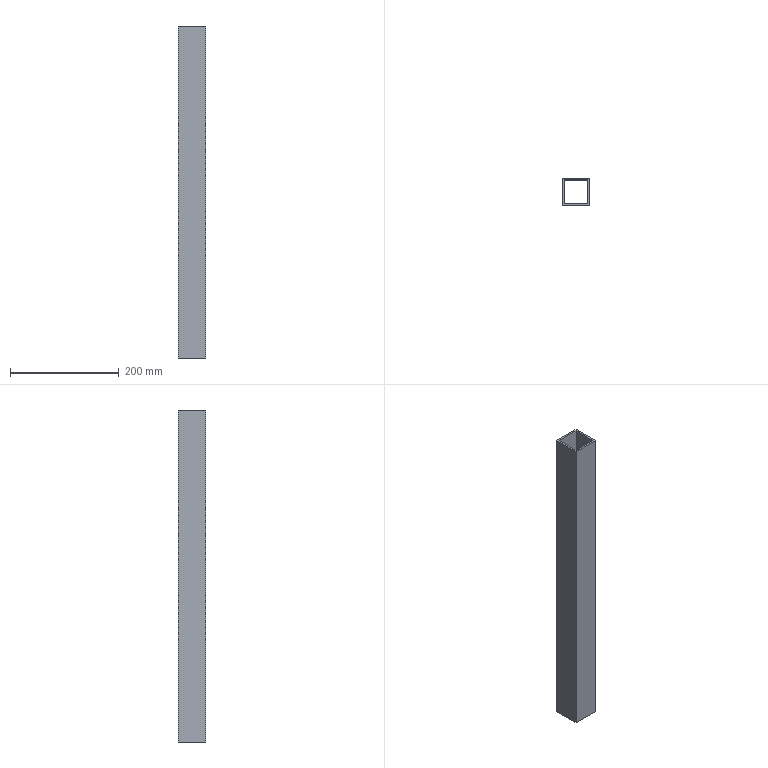Part | STEP file | BCC3 H19_2 | 1 solid | 10 faces | box 50 x 50 x 610 mm | volume 344040 mm3 | plane 10
STEP:
#1=CARTESIAN_POINT('',(0.,0.,0.));
#2=DIRECTION('',(0.,0.,1.));
#3=DIRECTION('',(1.,0.,0.));
#4=AXIS2_PLACEMENT_3D('',#1,#2,#3);
#5=CARTESIAN_POINT('',(-25.,25.,305.));
#6=VERTEX_POINT('',#5);
#7=CARTESIAN_POINT('',(-25.,-25.,305.));
#8=VERTEX_POINT('',#7);
#9=CARTESIAN_POINT('',(-25.,25.,305.));
#10=DIRECTION('',(0.,-1.,0.));
#11=VECTOR('',#10,1.);
#12=LINE('',#9,#11);
#13=CARTESIAN_POINT('',(0.,0.,305.));
#14=DIRECTION('',(0.,0.,1.));
#15=DIRECTION('',(1.,0.,0.));
#16=AXIS2_PLACEMENT_3D('',#13,#14,#15);
#17=PLANE('',#16);
#18=CARTESIAN_POINT('',(-25.,25.));
#19=DIRECTION('',(0.,-1.));
#20=VECTOR('',#19,1.);
#21=LINE('',#18,#20);
#22=(GEOMETRIC_REPRESENTATION_CONTEXT(2)PARAMETRIC_REPRESENTATION_CONTEXT()REPRESENTATION_CONTEXT('',''));
#23=DEFINITIONAL_REPRESENTATION('',(#21),#22);
#24=PCURVE('',#17,#23);
#25=CARTESIAN_POINT('',(-25.,25.,305.));
#26=DIRECTION('',(1.,0.,0.));
#27=DIRECTION('',(0.,1.,0.));
#28=AXIS2_PLACEMENT_3D('',#25,#26,#27);
#29=PLANE('',#28);
#30=CARTESIAN_POINT('',(0.,0.));
#31=DIRECTION('',(-1.,0.));
#32=VECTOR('',#31,1.);
#33=LINE('',#30,#32);
#34=(GEOMETRIC_REPRESENTATION_CONTEXT(2)PARAMETRIC_REPRESENTATION_CONTEXT()REPRESENTATION_CONTEXT('',''));
#35=DEFINITIONAL_REPRESENTATION('',(#33),#34);
#36=PCURVE('',#29,#35);
#37=SURFACE_CURVE('',#12,(#24,#36),.PCURVE_S1.);
#38=EDGE_CURVE('',#6,#8,#37,.T.);
#39=ORIENTED_EDGE('',*,*,#38,.T.);
#40=CARTESIAN_POINT('',(25.,-25.,305.));
#41=VERTEX_POINT('',#40);
#42=CARTESIAN_POINT('',(-25.,-25.,305.));
#43=DIRECTION('',(1.,0.,0.));
#44=VECTOR('',#43,1.);
#45=LINE('',#42,#44);
#46=CARTESIAN_POINT('',(-25.,-25.));
#47=DIRECTION('',(1.,0.));
#48=VECTOR('',#47,1.);
#49=LINE('',#46,#48);
#50=(GEOMETRIC_REPRESENTATION_CONTEXT(2)PARAMETRIC_REPRESENTATION_CONTEXT()REPRESENTATION_CONTEXT('',''));
#51=DEFINITIONAL_REPRESENTATION('',(#49),#50);
#52=PCURVE('',#17,#51);
#53=CARTESIAN_POINT('',(-25.,-25.,305.));
#54=DIRECTION('',(0.,1.,0.));
#55=DIRECTION('',(0.,0.,1.));
#56=AXIS2_PLACEMENT_3D('',#53,#54,#55);
#57=PLANE('',#56);
#58=CARTESIAN_POINT('',(0.,0.));
#59=DIRECTION('',(0.,1.));
#60=VECTOR('',#59,1.);
#61=LINE('',#58,#60);
#62=(GEOMETRIC_REPRESENTATION_CONTEXT(2)PARAMETRIC_REPRESENTATION_CONTEXT()REPRESENTATION_CONTEXT('',''));
#63=DEFINITIONAL_REPRESENTATION('',(#61),#62);
#64=PCURVE('',#57,#63);
#65=SURFACE_CURVE('',#45,(#52,#64),.PCURVE_S1.);
#66=EDGE_CURVE('',#8,#41,#65,.T.);
#67=ORIENTED_EDGE('',*,*,#66,.T.);
#68=CARTESIAN_POINT('',(25.,25.,305.));
#69=VERTEX_POINT('',#68);
#70=CARTESIAN_POINT('',(25.,25.,305.));
#71=DIRECTION('',(0.,1.,0.));
#72=VECTOR('',#71,1.);
#73=LINE('',#70,#72);
#74=CARTESIAN_POINT('',(25.,25.));
#75=DIRECTION('',(0.,1.));
#76=VECTOR('',#75,1.);
#77=LINE('',#74,#76);
#78=(GEOMETRIC_REPRESENTATION_CONTEXT(2)PARAMETRIC_REPRESENTATION_CONTEXT()REPRESENTATION_CONTEXT('',''));
#79=DEFINITIONAL_REPRESENTATION('',(#77),#78);
#80=PCURVE('',#17,#79);
#81=CARTESIAN_POINT('',(25.,25.,305.));
#82=DIRECTION('',(-1.,0.,0.));
#83=DIRECTION('',(0.,-1.,0.));
#84=AXIS2_PLACEMENT_3D('',#81,#82,#83);
#85=PLANE('',#84);
#86=CARTESIAN_POINT('',(0.,0.));
#87=DIRECTION('',(-1.,0.));
#88=VECTOR('',#87,1.);
#89=LINE('',#86,#88);
#90=(GEOMETRIC_REPRESENTATION_CONTEXT(2)PARAMETRIC_REPRESENTATION_CONTEXT()REPRESENTATION_CONTEXT('',''));
#91=DEFINITIONAL_REPRESENTATION('',(#89),#90);
#92=PCURVE('',#85,#91);
#93=SURFACE_CURVE('',#73,(#80,#92),.PCURVE_S1.);
#94=EDGE_CURVE('',#41,#69,#93,.T.);
#95=ORIENTED_EDGE('',*,*,#94,.T.);
#96=CARTESIAN_POINT('',(-25.,25.,305.));
#97=DIRECTION('',(-1.,0.,0.));
#98=VECTOR('',#97,1.);
#99=LINE('',#96,#98);
#100=CARTESIAN_POINT('',(-25.,25.));
#101=DIRECTION('',(-1.,0.));
#102=VECTOR('',#101,1.);
#103=LINE('',#100,#102);
#104=(GEOMETRIC_REPRESENTATION_CONTEXT(2)PARAMETRIC_REPRESENTATION_CONTEXT()REPRESENTATION_CONTEXT('',''));
#105=DEFINITIONAL_REPRESENTATION('',(#103),#104);
#106=PCURVE('',#17,#105);
#107=CARTESIAN_POINT('',(-25.,25.,305.));
#108=DIRECTION('',(0.,-1.,0.));
#109=DIRECTION('',(0.,0.,-1.));
#110=AXIS2_PLACEMENT_3D('',#107,#108,#109);
#111=PLANE('',#110);
#112=CARTESIAN_POINT('',(0.,0.));
#113=DIRECTION('',(0.,-1.));
#114=VECTOR('',#113,1.);
#115=LINE('',#112,#114);
#116=(GEOMETRIC_REPRESENTATION_CONTEXT(2)PARAMETRIC_REPRESENTATION_CONTEXT()REPRESENTATION_CONTEXT('',''));
#117=DEFINITIONAL_REPRESENTATION('',(#115),#116);
#118=PCURVE('',#111,#117);
#119=SURFACE_CURVE('',#99,(#106,#118),.PCURVE_S1.);
#120=EDGE_CURVE('',#69,#6,#119,.T.);
#121=ORIENTED_EDGE('',*,*,#120,.T.);
#122=EDGE_LOOP('',(#39,#67,#95,#121));
#123=FACE_BOUND('',#122,.T.);
#124=CARTESIAN_POINT('',(-22.,-22.,305.));
#125=VERTEX_POINT('',#124);
#126=CARTESIAN_POINT('',(22.,-22.,305.));
#127=VERTEX_POINT('',#126);
#128=CARTESIAN_POINT('',(-22.,-22.,305.));
#129=DIRECTION('',(1.,0.,0.));
#130=VECTOR('',#129,1.);
#131=LINE('',#128,#130);
#132=CARTESIAN_POINT('',(-22.,-22.));
#133=DIRECTION('',(1.,0.));
#134=VECTOR('',#133,1.);
#135=LINE('',#132,#134);
#136=(GEOMETRIC_REPRESENTATION_CONTEXT(2)PARAMETRIC_REPRESENTATION_CONTEXT()REPRESENTATION_CONTEXT('',''));
#137=DEFINITIONAL_REPRESENTATION('',(#135),#136);
#138=PCURVE('',#17,#137);
#139=CARTESIAN_POINT('',(-22.,-22.,305.));
#140=DIRECTION('',(0.,1.,0.));
#141=DIRECTION('',(-1.,0.,0.));
#142=AXIS2_PLACEMENT_3D('',#139,#140,#141);
#143=PLANE('',#142);
#144=CARTESIAN_POINT('',(0.,0.));
#145=DIRECTION('',(-1.,0.));
#146=VECTOR('',#145,1.);
#147=LINE('',#144,#146);
#148=(GEOMETRIC_REPRESENTATION_CONTEXT(2)PARAMETRIC_REPRESENTATION_CONTEXT()REPRESENTATION_CONTEXT('',''));
#149=DEFINITIONAL_REPRESENTATION('',(#147),#148);
#150=PCURVE('',#143,#149);
#151=SURFACE_CURVE('',#131,(#138,#150),.PCURVE_S1.);
#152=EDGE_CURVE('',#125,#127,#151,.T.);
#153=ORIENTED_EDGE('',*,*,#152,.F.);
#154=CARTESIAN_POINT('',(-22.,22.,305.));
#155=VERTEX_POINT('',#154);
#156=CARTESIAN_POINT('',(-22.,22.,305.));
#157=DIRECTION('',(0.,-1.,0.));
#158=VECTOR('',#157,1.);
#159=LINE('',#156,#158);
#160=CARTESIAN_POINT('',(-22.,22.));
#161=DIRECTION('',(0.,-1.));
#162=VECTOR('',#161,1.);
#163=LINE('',#160,#162);
#164=(GEOMETRIC_REPRESENTATION_CONTEXT(2)PARAMETRIC_REPRESENTATION_CONTEXT()REPRESENTATION_CONTEXT('',''));
#165=DEFINITIONAL_REPRESENTATION('',(#163),#164);
#166=PCURVE('',#17,#165);
#167=CARTESIAN_POINT('',(-22.,22.,305.));
#168=DIRECTION('',(1.,0.,0.));
#169=DIRECTION('',(0.,1.,0.));
#170=AXIS2_PLACEMENT_3D('',#167,#168,#169);
#171=PLANE('',#170);
#172=CARTESIAN_POINT('',(0.,0.));
#173=DIRECTION('',(-1.,0.));
#174=VECTOR('',#173,1.);
#175=LINE('',#172,#174);
#176=(GEOMETRIC_REPRESENTATION_CONTEXT(2)PARAMETRIC_REPRESENTATION_CONTEXT()REPRESENTATION_CONTEXT('',''));
#177=DEFINITIONAL_REPRESENTATION('',(#175),#176);
#178=PCURVE('',#171,#177);
#179=SURFACE_CURVE('',#159,(#166,#178),.PCURVE_S1.);
#180=EDGE_CURVE('',#155,#125,#179,.T.);
#181=ORIENTED_EDGE('',*,*,#180,.F.);
#182=CARTESIAN_POINT('',(22.,22.,305.));
#183=VERTEX_POINT('',#182);
#184=CARTESIAN_POINT('',(-22.,22.,305.));
#185=DIRECTION('',(-1.,0.,0.));
#186=VECTOR('',#185,1.);
#187=LINE('',#184,#186);
#188=CARTESIAN_POINT('',(-22.,22.));
#189=DIRECTION('',(-1.,0.));
#190=VECTOR('',#189,1.);
#191=LINE('',#188,#190);
#192=(GEOMETRIC_REPRESENTATION_CONTEXT(2)PARAMETRIC_REPRESENTATION_CONTEXT()REPRESENTATION_CONTEXT('',''));
#193=DEFINITIONAL_REPRESENTATION('',(#191),#192);
#194=PCURVE('',#17,#193);
#195=CARTESIAN_POINT('',(-22.,22.,305.));
#196=DIRECTION('',(0.,-1.,0.));
#197=DIRECTION('',(0.,0.,-1.));
#198=AXIS2_PLACEMENT_3D('',#195,#196,#197);
#199=PLANE('',#198);
#200=CARTESIAN_POINT('',(0.,0.));
#201=DIRECTION('',(0.,-1.));
#202=VECTOR('',#201,1.);
#203=LINE('',#200,#202);
#204=(GEOMETRIC_REPRESENTATION_CONTEXT(2)PARAMETRIC_REPRESENTATION_CONTEXT()REPRESENTATION_CONTEXT('',''));
#205=DEFINITIONAL_REPRESENTATION('',(#203),#204);
#206=PCURVE('',#199,#205);
#207=SURFACE_CURVE('',#187,(#194,#206),.PCURVE_S1.);
#208=EDGE_CURVE('',#183,#155,#207,.T.);
#209=ORIENTED_EDGE('',*,*,#208,.F.);
#210=CARTESIAN_POINT('',(22.,22.,305.));
#211=DIRECTION('',(0.,1.,0.));
#212=VECTOR('',#211,1.);
#213=LINE('',#210,#212);
#214=CARTESIAN_POINT('',(22.,22.));
#215=DIRECTION('',(0.,1.));
#216=VECTOR('',#215,1.);
#217=LINE('',#214,#216);
#218=(GEOMETRIC_REPRESENTATION_CONTEXT(2)PARAMETRIC_REPRESENTATION_CONTEXT()REPRESENTATION_CONTEXT('',''));
#219=DEFINITIONAL_REPRESENTATION('',(#217),#218);
#220=PCURVE('',#17,#219);
#221=CARTESIAN_POINT('',(22.,22.,305.));
#222=DIRECTION('',(-1.,0.,0.));
#223=DIRECTION('',(0.,-1.,0.));
#224=AXIS2_PLACEMENT_3D('',#221,#222,#223);
#225=PLANE('',#224);
#226=CARTESIAN_POINT('',(0.,0.));
#227=DIRECTION('',(-1.,0.));
#228=VECTOR('',#227,1.);
#229=LINE('',#226,#228);
#230=(GEOMETRIC_REPRESENTATION_CONTEXT(2)PARAMETRIC_REPRESENTATION_CONTEXT()REPRESENTATION_CONTEXT('',''));
#231=DEFINITIONAL_REPRESENTATION('',(#229),#230);
#232=PCURVE('',#225,#231);
#233=SURFACE_CURVE('',#213,(#220,#232),.PCURVE_S1.);
#234=EDGE_CURVE('',#127,#183,#233,.T.);
#235=ORIENTED_EDGE('',*,*,#234,.F.);
#236=EDGE_LOOP('',(#153,#181,#209,#235));
#237=FACE_BOUND('',#236,.T.);
#238=ADVANCED_FACE('',(#123,#237),#17,.T.);
#239=CARTESIAN_POINT('',(-25.,25.,-305.));
#240=VERTEX_POINT('',#239);
#241=CARTESIAN_POINT('',(-25.,-25.,-305.));
#242=VERTEX_POINT('',#241);
#243=CARTESIAN_POINT('',(-25.,25.,-305.));
#244=DIRECTION('',(0.,-1.,0.));
#245=VECTOR('',#244,1.);
#246=LINE('',#243,#245);
#247=CARTESIAN_POINT('',(0.,0.,-305.));
#248=DIRECTION('',(0.,0.,1.));
#249=DIRECTION('',(1.,0.,0.));
#250=AXIS2_PLACEMENT_3D('',#247,#248,#249);
#251=PLANE('',#250);
#252=CARTESIAN_POINT('',(-25.,25.));
#253=DIRECTION('',(0.,-1.));
#254=VECTOR('',#253,1.);
#255=LINE('',#252,#254);
#256=(GEOMETRIC_REPRESENTATION_CONTEXT(2)PARAMETRIC_REPRESENTATION_CONTEXT()REPRESENTATION_CONTEXT('',''));
#257=DEFINITIONAL_REPRESENTATION('',(#255),#256);
#258=PCURVE('',#251,#257);
#259=CARTESIAN_POINT('',(0.,-610.));
#260=DIRECTION('',(-1.,0.));
#261=VECTOR('',#260,1.);
#262=LINE('',#259,#261);
#263=(GEOMETRIC_REPRESENTATION_CONTEXT(2)PARAMETRIC_REPRESENTATION_CONTEXT()REPRESENTATION_CONTEXT('',''));
#264=DEFINITIONAL_REPRESENTATION('',(#262),#263);
#265=PCURVE('',#29,#264);
#266=SURFACE_CURVE('',#246,(#258,#265),.PCURVE_S1.);
#267=EDGE_CURVE('',#240,#242,#266,.T.);
#268=ORIENTED_EDGE('',*,*,#267,.F.);
#269=CARTESIAN_POINT('',(25.,25.,-305.));
#270=VERTEX_POINT('',#269);
#271=CARTESIAN_POINT('',(-25.,25.,-305.));
#272=DIRECTION('',(-1.,0.,0.));
#273=VECTOR('',#272,1.);
#274=LINE('',#271,#273);
#275=CARTESIAN_POINT('',(-25.,25.));
#276=DIRECTION('',(-1.,0.));
#277=VECTOR('',#276,1.);
#278=LINE('',#275,#277);
#279=(GEOMETRIC_REPRESENTATION_CONTEXT(2)PARAMETRIC_REPRESENTATION_CONTEXT()REPRESENTATION_CONTEXT('',''));
#280=DEFINITIONAL_REPRESENTATION('',(#278),#279);
#281=PCURVE('',#251,#280);
#282=CARTESIAN_POINT('',(610.,0.));
#283=DIRECTION('',(0.,-1.));
#284=VECTOR('',#283,1.);
#285=LINE('',#282,#284);
#286=(GEOMETRIC_REPRESENTATION_CONTEXT(2)PARAMETRIC_REPRESENTATION_CONTEXT()REPRESENTATION_CONTEXT('',''));
#287=DEFINITIONAL_REPRESENTATION('',(#285),#286);
#288=PCURVE('',#111,#287);
#289=SURFACE_CURVE('',#274,(#281,#288),.PCURVE_S1.);
#290=EDGE_CURVE('',#270,#240,#289,.T.);
#291=ORIENTED_EDGE('',*,*,#290,.F.);
#292=CARTESIAN_POINT('',(25.,-25.,-305.));
#293=VERTEX_POINT('',#292);
#294=CARTESIAN_POINT('',(25.,25.,-305.));
#295=DIRECTION('',(0.,1.,0.));
#296=VECTOR('',#295,1.);
#297=LINE('',#294,#296);
#298=CARTESIAN_POINT('',(25.,25.));
#299=DIRECTION('',(0.,1.));
#300=VECTOR('',#299,1.);
#301=LINE('',#298,#300);
#302=(GEOMETRIC_REPRESENTATION_CONTEXT(2)PARAMETRIC_REPRESENTATION_CONTEXT()REPRESENTATION_CONTEXT('',''));
#303=DEFINITIONAL_REPRESENTATION('',(#301),#302);
#304=PCURVE('',#251,#303);
#305=CARTESIAN_POINT('',(0.,-610.));
#306=DIRECTION('',(-1.,0.));
#307=VECTOR('',#306,1.);
#308=LINE('',#305,#307);
#309=(GEOMETRIC_REPRESENTATION_CONTEXT(2)PARAMETRIC_REPRESENTATION_CONTEXT()REPRESENTATION_CONTEXT('',''));
#310=DEFINITIONAL_REPRESENTATION('',(#308),#309);
#311=PCURVE('',#85,#310);
#312=SURFACE_CURVE('',#297,(#304,#311),.PCURVE_S1.);
#313=EDGE_CURVE('',#293,#270,#312,.T.);
#314=ORIENTED_EDGE('',*,*,#313,.F.);
#315=CARTESIAN_POINT('',(-25.,-25.,-305.));
#316=DIRECTION('',(1.,0.,0.));
#317=VECTOR('',#316,1.);
#318=LINE('',#315,#317);
#319=CARTESIAN_POINT('',(-25.,-25.));
#320=DIRECTION('',(1.,0.));
#321=VECTOR('',#320,1.);
#322=LINE('',#319,#321);
#323=(GEOMETRIC_REPRESENTATION_CONTEXT(2)PARAMETRIC_REPRESENTATION_CONTEXT()REPRESENTATION_CONTEXT('',''));
#324=DEFINITIONAL_REPRESENTATION('',(#322),#323);
#325=PCURVE('',#251,#324);
#326=CARTESIAN_POINT('',(-610.,0.));
#327=DIRECTION('',(0.,1.));
#328=VECTOR('',#327,1.);
#329=LINE('',#326,#328);
#330=(GEOMETRIC_REPRESENTATION_CONTEXT(2)PARAMETRIC_REPRESENTATION_CONTEXT()REPRESENTATION_CONTEXT('',''));
#331=DEFINITIONAL_REPRESENTATION('',(#329),#330);
#332=PCURVE('',#57,#331);
#333=SURFACE_CURVE('',#318,(#325,#332),.PCURVE_S1.);
#334=EDGE_CURVE('',#242,#293,#333,.T.);
#335=ORIENTED_EDGE('',*,*,#334,.F.);
#336=EDGE_LOOP('',(#268,#291,#314,#335));
#337=FACE_BOUND('',#336,.T.);
#338=CARTESIAN_POINT('',(-22.,22.,-305.));
#339=VERTEX_POINT('',#338);
#340=CARTESIAN_POINT('',(-22.,-22.,-305.));
#341=VERTEX_POINT('',#340);
#342=CARTESIAN_POINT('',(-22.,22.,-305.));
#343=DIRECTION('',(0.,-1.,0.));
#344=VECTOR('',#343,1.);
#345=LINE('',#342,#344);
#346=CARTESIAN_POINT('',(-22.,22.));
#347=DIRECTION('',(0.,-1.));
#348=VECTOR('',#347,1.);
#349=LINE('',#346,#348);
#350=(GEOMETRIC_REPRESENTATION_CONTEXT(2)PARAMETRIC_REPRESENTATION_CONTEXT()REPRESENTATION_CONTEXT('',''));
#351=DEFINITIONAL_REPRESENTATION('',(#349),#350);
#352=PCURVE('',#251,#351);
#353=CARTESIAN_POINT('',(0.,-610.));
#354=DIRECTION('',(-1.,0.));
#355=VECTOR('',#354,1.);
#356=LINE('',#353,#355);
#357=(GEOMETRIC_REPRESENTATION_CONTEXT(2)PARAMETRIC_REPRESENTATION_CONTEXT()REPRESENTATION_CONTEXT('',''));
#358=DEFINITIONAL_REPRESENTATION('',(#356),#357);
#359=PCURVE('',#171,#358);
#360=SURFACE_CURVE('',#345,(#352,#359),.PCURVE_S1.);
#361=EDGE_CURVE('',#339,#341,#360,.T.);
#362=ORIENTED_EDGE('',*,*,#361,.T.);
#363=CARTESIAN_POINT('',(22.,-22.,-305.));
#364=VERTEX_POINT('',#363);
#365=CARTESIAN_POINT('',(-22.,-22.,-305.));
#366=DIRECTION('',(1.,0.,0.));
#367=VECTOR('',#366,1.);
#368=LINE('',#365,#367);
#369=CARTESIAN_POINT('',(-22.,-22.));
#370=DIRECTION('',(1.,0.));
#371=VECTOR('',#370,1.);
#372=LINE('',#369,#371);
#373=(GEOMETRIC_REPRESENTATION_CONTEXT(2)PARAMETRIC_REPRESENTATION_CONTEXT()REPRESENTATION_CONTEXT('',''));
#374=DEFINITIONAL_REPRESENTATION('',(#372),#373);
#375=PCURVE('',#251,#374);
#376=CARTESIAN_POINT('',(0.,-610.));
#377=DIRECTION('',(-1.,0.));
#378=VECTOR('',#377,1.);
#379=LINE('',#376,#378);
#380=(GEOMETRIC_REPRESENTATION_CONTEXT(2)PARAMETRIC_REPRESENTATION_CONTEXT()REPRESENTATION_CONTEXT('',''));
#381=DEFINITIONAL_REPRESENTATION('',(#379),#380);
#382=PCURVE('',#143,#381);
#383=SURFACE_CURVE('',#368,(#375,#382),.PCURVE_S1.);
#384=EDGE_CURVE('',#341,#364,#383,.T.);
#385=ORIENTED_EDGE('',*,*,#384,.T.);
#386=CARTESIAN_POINT('',(22.,22.,-305.));
#387=VERTEX_POINT('',#386);
#388=CARTESIAN_POINT('',(22.,22.,-305.));
#389=DIRECTION('',(0.,1.,0.));
#390=VECTOR('',#389,1.);
#391=LINE('',#388,#390);
#392=CARTESIAN_POINT('',(22.,22.));
#393=DIRECTION('',(0.,1.));
#394=VECTOR('',#393,1.);
#395=LINE('',#392,#394);
#396=(GEOMETRIC_REPRESENTATION_CONTEXT(2)PARAMETRIC_REPRESENTATION_CONTEXT()REPRESENTATION_CONTEXT('',''));
#397=DEFINITIONAL_REPRESENTATION('',(#395),#396);
#398=PCURVE('',#251,#397);
#399=CARTESIAN_POINT('',(0.,-610.));
#400=DIRECTION('',(-1.,0.));
#401=VECTOR('',#400,1.);
#402=LINE('',#399,#401);
#403=(GEOMETRIC_REPRESENTATION_CONTEXT(2)PARAMETRIC_REPRESENTATION_CONTEXT()REPRESENTATION_CONTEXT('',''));
#404=DEFINITIONAL_REPRESENTATION('',(#402),#403);
#405=PCURVE('',#225,#404);
#406=SURFACE_CURVE('',#391,(#398,#405),.PCURVE_S1.);
#407=EDGE_CURVE('',#364,#387,#406,.T.);
#408=ORIENTED_EDGE('',*,*,#407,.T.);
#409=CARTESIAN_POINT('',(-22.,22.,-305.));
#410=DIRECTION('',(-1.,0.,0.));
#411=VECTOR('',#410,1.);
#412=LINE('',#409,#411);
#413=CARTESIAN_POINT('',(-22.,22.));
#414=DIRECTION('',(-1.,0.));
#415=VECTOR('',#414,1.);
#416=LINE('',#413,#415);
#417=(GEOMETRIC_REPRESENTATION_CONTEXT(2)PARAMETRIC_REPRESENTATION_CONTEXT()REPRESENTATION_CONTEXT('',''));
#418=DEFINITIONAL_REPRESENTATION('',(#416),#417);
#419=PCURVE('',#251,#418);
#420=CARTESIAN_POINT('',(610.,0.));
#421=DIRECTION('',(0.,-1.));
#422=VECTOR('',#421,1.);
#423=LINE('',#420,#422);
#424=(GEOMETRIC_REPRESENTATION_CONTEXT(2)PARAMETRIC_REPRESENTATION_CONTEXT()REPRESENTATION_CONTEXT('',''));
#425=DEFINITIONAL_REPRESENTATION('',(#423),#424);
#426=PCURVE('',#199,#425);
#427=SURFACE_CURVE('',#412,(#419,#426),.PCURVE_S1.);
#428=EDGE_CURVE('',#387,#339,#427,.T.);
#429=ORIENTED_EDGE('',*,*,#428,.T.);
#430=EDGE_LOOP('',(#362,#385,#408,#429));
#431=FACE_BOUND('',#430,.T.);
#432=ADVANCED_FACE('',(#337,#431),#251,.F.);
#433=ORIENTED_EDGE('',*,*,#267,.T.);
#434=CARTESIAN_POINT('',(-25.,-25.,305.));
#435=DIRECTION('',(0.,0.,-1.));
#436=VECTOR('',#435,1.);
#437=LINE('',#434,#436);
#438=CARTESIAN_POINT('',(-50.,0.));
#439=DIRECTION('',(0.,-1.));
#440=VECTOR('',#439,1.);
#441=LINE('',#438,#440);
#442=(GEOMETRIC_REPRESENTATION_CONTEXT(2)PARAMETRIC_REPRESENTATION_CONTEXT()REPRESENTATION_CONTEXT('',''));
#443=DEFINITIONAL_REPRESENTATION('',(#441),#442);
#444=PCURVE('',#29,#443);
#445=CARTESIAN_POINT('',(0.,0.));
#446=DIRECTION('',(-1.,0.));
#447=VECTOR('',#446,1.);
#448=LINE('',#445,#447);
#449=(GEOMETRIC_REPRESENTATION_CONTEXT(2)PARAMETRIC_REPRESENTATION_CONTEXT()REPRESENTATION_CONTEXT('',''));
#450=DEFINITIONAL_REPRESENTATION('',(#448),#449);
#451=PCURVE('',#57,#450);
#452=SURFACE_CURVE('',#437,(#444,#451),.PCURVE_S1.);
#453=EDGE_CURVE('',#8,#242,#452,.T.);
#454=ORIENTED_EDGE('',*,*,#453,.F.);
#455=ORIENTED_EDGE('',*,*,#38,.F.);
#456=CARTESIAN_POINT('',(-25.,25.,305.));
#457=DIRECTION('',(0.,0.,-1.));
#458=VECTOR('',#457,1.);
#459=LINE('',#456,#458);
#460=CARTESIAN_POINT('',(0.,0.));
#461=DIRECTION('',(0.,-1.));
#462=VECTOR('',#461,1.);
#463=LINE('',#460,#462);
#464=(GEOMETRIC_REPRESENTATION_CONTEXT(2)PARAMETRIC_REPRESENTATION_CONTEXT()REPRESENTATION_CONTEXT('',''));
#465=DEFINITIONAL_REPRESENTATION('',(#463),#464);
#466=PCURVE('',#29,#465);
#467=CARTESIAN_POINT('',(0.,0.));
#468=DIRECTION('',(1.,0.));
#469=VECTOR('',#468,1.);
#470=LINE('',#467,#469);
#471=(GEOMETRIC_REPRESENTATION_CONTEXT(2)PARAMETRIC_REPRESENTATION_CONTEXT()REPRESENTATION_CONTEXT('',''));
#472=DEFINITIONAL_REPRESENTATION('',(#470),#471);
#473=PCURVE('',#111,#472);
#474=SURFACE_CURVE('',#459,(#466,#473),.PCURVE_S1.);
#475=EDGE_CURVE('',#6,#240,#474,.T.);
#476=ORIENTED_EDGE('',*,*,#475,.T.);
#477=EDGE_LOOP('',(#433,#454,#455,#476));
#478=FACE_BOUND('',#477,.T.);
#479=ADVANCED_FACE('',(#478),#29,.F.);
#480=ORIENTED_EDGE('',*,*,#334,.T.);
#481=CARTESIAN_POINT('',(25.,-25.,305.));
#482=DIRECTION('',(0.,0.,-1.));
#483=VECTOR('',#482,1.);
#484=LINE('',#481,#483);
#485=CARTESIAN_POINT('',(0.,50.));
#486=DIRECTION('',(-1.,0.));
#487=VECTOR('',#486,1.);
#488=LINE('',#485,#487);
#489=(GEOMETRIC_REPRESENTATION_CONTEXT(2)PARAMETRIC_REPRESENTATION_CONTEXT()REPRESENTATION_CONTEXT('',''));
#490=DEFINITIONAL_REPRESENTATION('',(#488),#489);
#491=PCURVE('',#57,#490);
#492=CARTESIAN_POINT('',(50.,0.));
#493=DIRECTION('',(0.,-1.));
#494=VECTOR('',#493,1.);
#495=LINE('',#492,#494);
#496=(GEOMETRIC_REPRESENTATION_CONTEXT(2)PARAMETRIC_REPRESENTATION_CONTEXT()REPRESENTATION_CONTEXT('',''));
#497=DEFINITIONAL_REPRESENTATION('',(#495),#496);
#498=PCURVE('',#85,#497);
#499=SURFACE_CURVE('',#484,(#491,#498),.PCURVE_S1.);
#500=EDGE_CURVE('',#41,#293,#499,.T.);
#501=ORIENTED_EDGE('',*,*,#500,.F.);
#502=ORIENTED_EDGE('',*,*,#66,.F.);
#503=ORIENTED_EDGE('',*,*,#453,.T.);
#504=EDGE_LOOP('',(#480,#501,#502,#503));
#505=FACE_BOUND('',#504,.T.);
#506=ADVANCED_FACE('',(#505),#57,.F.);
#507=ORIENTED_EDGE('',*,*,#313,.T.);
#508=CARTESIAN_POINT('',(25.,25.,305.));
#509=DIRECTION('',(0.,0.,-1.));
#510=VECTOR('',#509,1.);
#511=LINE('',#508,#510);
#512=CARTESIAN_POINT('',(0.,0.));
#513=DIRECTION('',(0.,-1.));
#514=VECTOR('',#513,1.);
#515=LINE('',#512,#514);
#516=(GEOMETRIC_REPRESENTATION_CONTEXT(2)PARAMETRIC_REPRESENTATION_CONTEXT()REPRESENTATION_CONTEXT('',''));
#517=DEFINITIONAL_REPRESENTATION('',(#515),#516);
#518=PCURVE('',#85,#517);
#519=CARTESIAN_POINT('',(0.,50.));
#520=DIRECTION('',(1.,0.));
#521=VECTOR('',#520,1.);
#522=LINE('',#519,#521);
#523=(GEOMETRIC_REPRESENTATION_CONTEXT(2)PARAMETRIC_REPRESENTATION_CONTEXT()REPRESENTATION_CONTEXT('',''));
#524=DEFINITIONAL_REPRESENTATION('',(#522),#523);
#525=PCURVE('',#111,#524);
#526=SURFACE_CURVE('',#511,(#518,#525),.PCURVE_S1.);
#527=EDGE_CURVE('',#69,#270,#526,.T.);
#528=ORIENTED_EDGE('',*,*,#527,.F.);
#529=ORIENTED_EDGE('',*,*,#94,.F.);
#530=ORIENTED_EDGE('',*,*,#500,.T.);
#531=EDGE_LOOP('',(#507,#528,#529,#530));
#532=FACE_BOUND('',#531,.T.);
#533=ADVANCED_FACE('',(#532),#85,.F.);
#534=ORIENTED_EDGE('',*,*,#290,.T.);
#535=ORIENTED_EDGE('',*,*,#475,.F.);
#536=ORIENTED_EDGE('',*,*,#120,.F.);
#537=ORIENTED_EDGE('',*,*,#527,.T.);
#538=EDGE_LOOP('',(#534,#535,#536,#537));
#539=FACE_BOUND('',#538,.T.);
#540=ADVANCED_FACE('',(#539),#111,.F.);
#541=ORIENTED_EDGE('',*,*,#361,.F.);
#542=CARTESIAN_POINT('',(-22.,22.,305.));
#543=DIRECTION('',(0.,0.,-1.));
#544=VECTOR('',#543,1.);
#545=LINE('',#542,#544);
#546=CARTESIAN_POINT('',(0.,0.));
#547=DIRECTION('',(0.,-1.));
#548=VECTOR('',#547,1.);
#549=LINE('',#546,#548);
#550=(GEOMETRIC_REPRESENTATION_CONTEXT(2)PARAMETRIC_REPRESENTATION_CONTEXT()REPRESENTATION_CONTEXT('',''));
#551=DEFINITIONAL_REPRESENTATION('',(#549),#550);
#552=PCURVE('',#171,#551);
#553=CARTESIAN_POINT('',(0.,0.));
#554=DIRECTION('',(1.,0.));
#555=VECTOR('',#554,1.);
#556=LINE('',#553,#555);
#557=(GEOMETRIC_REPRESENTATION_CONTEXT(2)PARAMETRIC_REPRESENTATION_CONTEXT()REPRESENTATION_CONTEXT('',''));
#558=DEFINITIONAL_REPRESENTATION('',(#556),#557);
#559=PCURVE('',#199,#558);
#560=SURFACE_CURVE('',#545,(#552,#559),.PCURVE_S1.);
#561=EDGE_CURVE('',#155,#339,#560,.T.);
#562=ORIENTED_EDGE('',*,*,#561,.F.);
#563=ORIENTED_EDGE('',*,*,#180,.T.);
#564=CARTESIAN_POINT('',(-22.,-22.,305.));
#565=DIRECTION('',(0.,0.,-1.));
#566=VECTOR('',#565,1.);
#567=LINE('',#564,#566);
#568=CARTESIAN_POINT('',(-44.,0.));
#569=DIRECTION('',(0.,-1.));
#570=VECTOR('',#569,1.);
#571=LINE('',#568,#570);
#572=(GEOMETRIC_REPRESENTATION_CONTEXT(2)PARAMETRIC_REPRESENTATION_CONTEXT()REPRESENTATION_CONTEXT('',''));
#573=DEFINITIONAL_REPRESENTATION('',(#571),#572);
#574=PCURVE('',#171,#573);
#575=CARTESIAN_POINT('',(0.,0.));
#576=DIRECTION('',(0.,-1.));
#577=VECTOR('',#576,1.);
#578=LINE('',#575,#577);
#579=(GEOMETRIC_REPRESENTATION_CONTEXT(2)PARAMETRIC_REPRESENTATION_CONTEXT()REPRESENTATION_CONTEXT('',''));
#580=DEFINITIONAL_REPRESENTATION('',(#578),#579);
#581=PCURVE('',#143,#580);
#582=SURFACE_CURVE('',#567,(#574,#581),.PCURVE_S1.);
#583=EDGE_CURVE('',#125,#341,#582,.T.);
#584=ORIENTED_EDGE('',*,*,#583,.T.);
#585=EDGE_LOOP('',(#541,#562,#563,#584));
#586=FACE_BOUND('',#585,.T.);
#587=ADVANCED_FACE('',(#586),#171,.T.);
#588=ORIENTED_EDGE('',*,*,#384,.F.);
#589=ORIENTED_EDGE('',*,*,#583,.F.);
#590=ORIENTED_EDGE('',*,*,#152,.T.);
#591=CARTESIAN_POINT('',(22.,-22.,305.));
#592=DIRECTION('',(0.,0.,-1.));
#593=VECTOR('',#592,1.);
#594=LINE('',#591,#593);
#595=CARTESIAN_POINT('',(-44.,0.));
#596=DIRECTION('',(0.,-1.));
#597=VECTOR('',#596,1.);
#598=LINE('',#595,#597);
#599=(GEOMETRIC_REPRESENTATION_CONTEXT(2)PARAMETRIC_REPRESENTATION_CONTEXT()REPRESENTATION_CONTEXT('',''));
#600=DEFINITIONAL_REPRESENTATION('',(#598),#599);
#601=PCURVE('',#143,#600);
#602=CARTESIAN_POINT('',(44.,0.));
#603=DIRECTION('',(0.,-1.));
#604=VECTOR('',#603,1.);
#605=LINE('',#602,#604);
#606=(GEOMETRIC_REPRESENTATION_CONTEXT(2)PARAMETRIC_REPRESENTATION_CONTEXT()REPRESENTATION_CONTEXT('',''));
#607=DEFINITIONAL_REPRESENTATION('',(#605),#606);
#608=PCURVE('',#225,#607);
#609=SURFACE_CURVE('',#594,(#601,#608),.PCURVE_S1.);
#610=EDGE_CURVE('',#127,#364,#609,.T.);
#611=ORIENTED_EDGE('',*,*,#610,.T.);
#612=EDGE_LOOP('',(#588,#589,#590,#611));
#613=FACE_BOUND('',#612,.T.);
#614=ADVANCED_FACE('',(#613),#143,.T.);
#615=ORIENTED_EDGE('',*,*,#407,.F.);
#616=ORIENTED_EDGE('',*,*,#610,.F.);
#617=ORIENTED_EDGE('',*,*,#234,.T.);
#618=CARTESIAN_POINT('',(22.,22.,305.));
#619=DIRECTION('',(0.,0.,-1.));
#620=VECTOR('',#619,1.);
#621=LINE('',#618,#620);
#622=CARTESIAN_POINT('',(0.,0.));
#623=DIRECTION('',(0.,-1.));
#624=VECTOR('',#623,1.);
#625=LINE('',#622,#624);
#626=(GEOMETRIC_REPRESENTATION_CONTEXT(2)PARAMETRIC_REPRESENTATION_CONTEXT()REPRESENTATION_CONTEXT('',''));
#627=DEFINITIONAL_REPRESENTATION('',(#625),#626);
#628=PCURVE('',#225,#627);
#629=CARTESIAN_POINT('',(0.,44.));
#630=DIRECTION('',(1.,0.));
#631=VECTOR('',#630,1.);
#632=LINE('',#629,#631);
#633=(GEOMETRIC_REPRESENTATION_CONTEXT(2)PARAMETRIC_REPRESENTATION_CONTEXT()REPRESENTATION_CONTEXT('',''));
#634=DEFINITIONAL_REPRESENTATION('',(#632),#633);
#635=PCURVE('',#199,#634);
#636=SURFACE_CURVE('',#621,(#628,#635),.PCURVE_S1.);
#637=EDGE_CURVE('',#183,#387,#636,.T.);
#638=ORIENTED_EDGE('',*,*,#637,.T.);
#639=EDGE_LOOP('',(#615,#616,#617,#638));
#640=FACE_BOUND('',#639,.T.);
#641=ADVANCED_FACE('',(#640),#225,.T.);
#642=ORIENTED_EDGE('',*,*,#428,.F.);
#643=ORIENTED_EDGE('',*,*,#637,.F.);
#644=ORIENTED_EDGE('',*,*,#208,.T.);
#645=ORIENTED_EDGE('',*,*,#561,.T.);
#646=EDGE_LOOP('',(#642,#643,#644,#645));
#647=FACE_BOUND('',#646,.T.);
#648=ADVANCED_FACE('',(#647),#199,.T.);
#649=CLOSED_SHELL('',(#238,#432,#479,#506,#533,#540,#587,#614,#641,#648));
#650=MANIFOLD_SOLID_BREP('',#649);
#651=(LENGTH_UNIT()NAMED_UNIT(*)SI_UNIT(.MILLI.,.METRE.));
#652=UNCERTAINTY_MEASURE_WITH_UNIT(LENGTH_MEASURE(0.0000001),#651,'','');
#653=(NAMED_UNIT(*)PLANE_ANGLE_UNIT()SI_UNIT($,.RADIAN.));
#654=(NAMED_UNIT(*)SI_UNIT($,.STERADIAN.)SOLID_ANGLE_UNIT());
#655=(GEOMETRIC_REPRESENTATION_CONTEXT(3)GLOBAL_UNCERTAINTY_ASSIGNED_CONTEXT((#652))GLOBAL_UNIT_ASSIGNED_CONTEXT((#651,#653,#654))REPRESENTATION_CONTEXT('',''));
#656=ADVANCED_BREP_SHAPE_REPRESENTATION('',(#4,#650),#655);